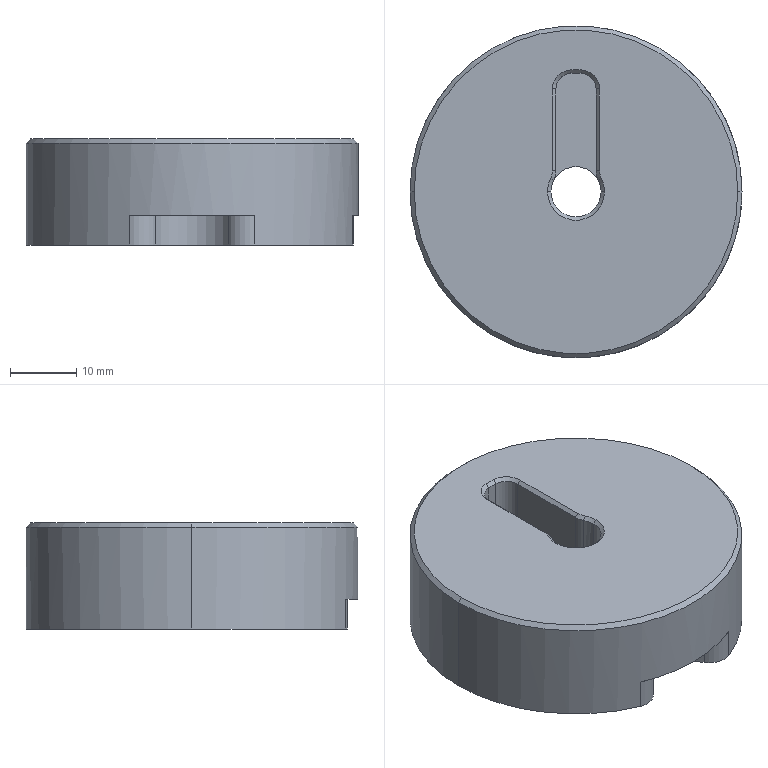CAM job | NX | 3-axis milling, drilling | part box 50.292 x 50.292 x 16.057 mm | stock box 50.292 x 50.292 x 16.057 mm
Tools:
number,name,description,diameter,corner_radius,flute_length,length,flutes
4,D4,Milling Tool-5 Parameters,4.0,0.0,50.0,75.0,2
5,D4JING,Milling Tool-5 Parameters,4.0,0.0,50.0,75.0,2
3,D4_CHAMFER-MILL,Milling Tool-5 Parameters,2.0,0.0,1.0,1.0,2
1,ZXZ,Milling Tool-5 Parameters,6.0,0.0,50.0,75.0,2
Operations:
program,operation,operation_type,tool,method,geometry_group,spindle_rpm,surface_speed,feed_per_tooth,feed_cut,feed_plunge,cut_length_mm,path_length_mm,cut_time_min,machine_time_min
1,ZLEVEL_PROFILE_COPY_1,ZLevelMilling,D4,METHOD,A,4000.0,50.0,0.1875,1500.0,1000.0,1921.6,2098.335,1.301,1.319
1,ZLEVEL_PROFILE_COPY_COPY_1_COPY_COPY_COPY_1,ZLevelMilling,D4JING,METHOD,A,4000.0,50.0,0.1062,850.0,100.0,34.975,117.201,0.0411,0.0494
1,PLANAR_MILL,PlanarMilling,D4_CHAMFER-MILL,METHOD,A,4000.0,25.0,0.125,1000.0,100.0,93.894,152.494,0.0939,0.0998
2,DRILLING_COPY_1,Operation,ZXZ,METHOD,B,3000.0,56.0,0.0333,200.0,0.0,12.0,133.574,0.06,0.0722
2,FLOOR_WALL_1,VolumeBased25DMillingOperation,D4,METHOD,B,4000.0,50.0,0.225,1800.0,100.0,3727.085,4044.442,2.071,2.102
2,FLOOR_WALL_1_COPY,VolumeBased25DMillingOperation,D4JING,METHOD,B,5000.0,31.0,0.1,1000.0,100.0,231.333,506.346,0.2313,0.2588
2,PLANAR_MILL_COPY,PlanarMilling,D4_CHAMFER-MILL,METHOD,B,4000.0,25.0,0.125,1000.0,100.0,70.131,208.937,0.0701,0.084
2,PLANAR_MILL_COPY_COPY,PlanarMilling,D4_CHAMFER-MILL,METHOD,B,4000.0,25.0,0.125,1000.0,100.0,42.047,227.981,0.042,0.0606